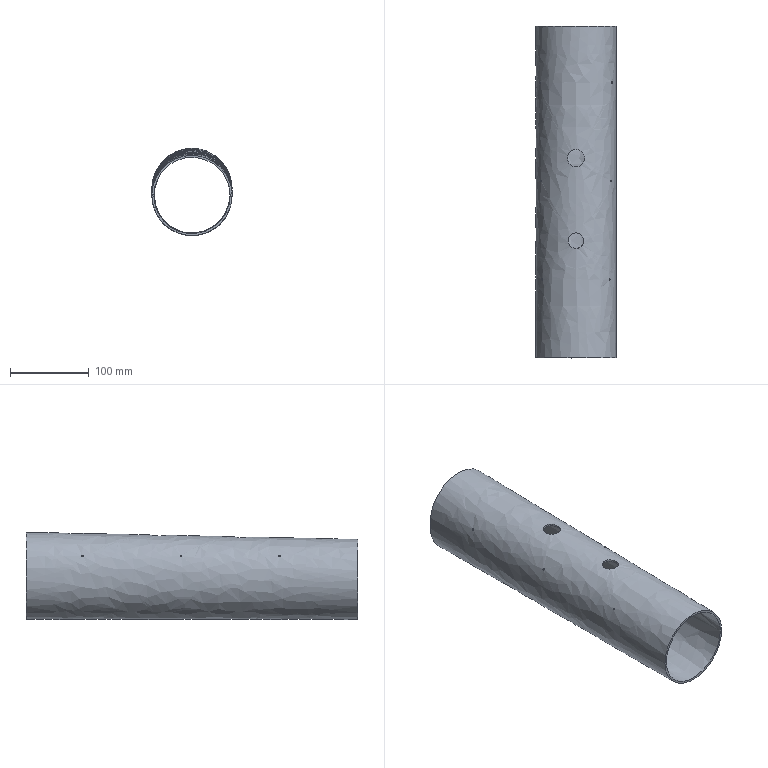Part | STEP file | 1-56.4 | 1 solid | 12 faces | box 102.005 x 421.966 x 111 mm | volume 341502 mm3 | cylinder 8 | plane 2 | spline 2 | commonest cylinder face diameters 2 x6 20 x1 22 x1